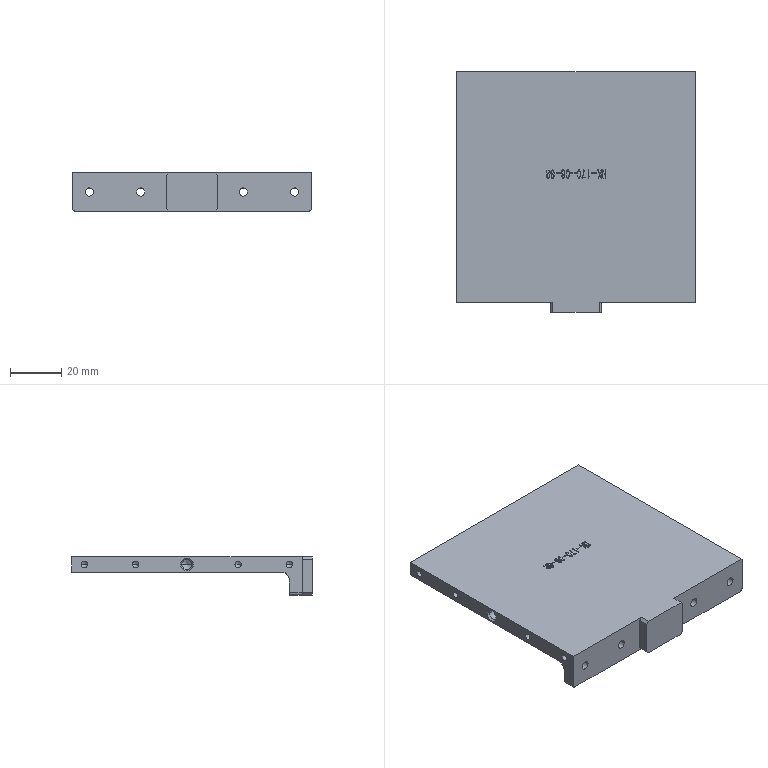Part | 1 solid | 286 faces | box 93.2 x 94 x 15 mm | volume 39361 mm3 | plane 132 | spline 87 | cylinder 39 | cone 28 | commonest cylinder face diameters 2.5 x16 3.3 x8 6 x5 4 x4 10 x4 2 x2